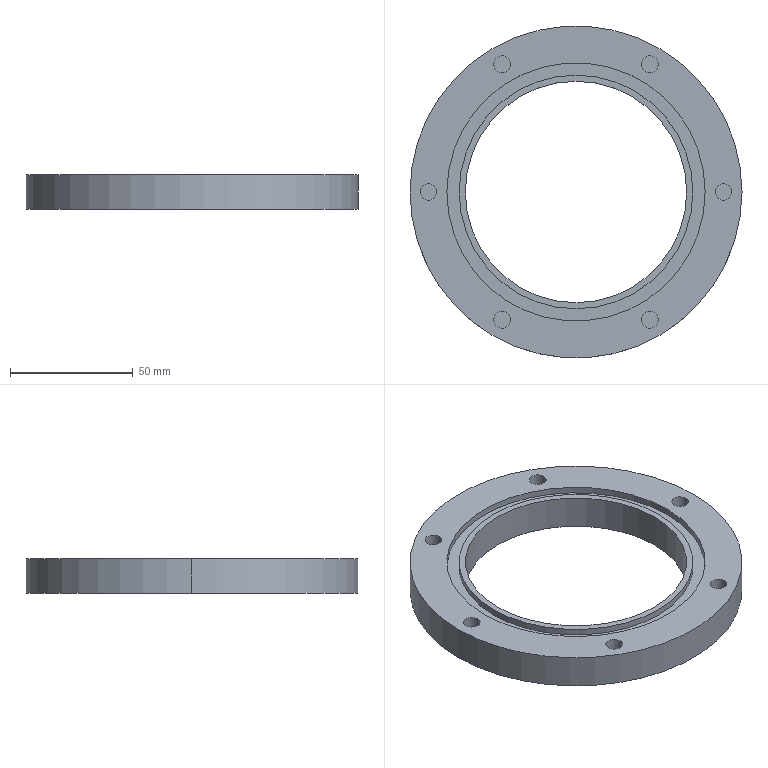Part | SolidWorks | features ICE 2, CirPattern 1, FlatPattern 1, HoleWzd 1, SMBaseFlange 1, SheetMetal 1 | 1 solid | 30 faces | box 135 x 135 x 14 mm | volume 104256 mm3 | cylinder 20 | plane 10 | commonest cylinder face diameters 6.8 x12 90 x2 95 x2 105 x2 135 x2
STEP:
#1=CARTESIAN_POINT('',(47.5,0.,-2.7));
#2=VERTEX_POINT('',#1);
#3=CARTESIAN_POINT('',(-47.5,0.,-2.7));
#4=VERTEX_POINT('',#3);
#5=CARTESIAN_POINT('',(0.,0.,-2.7));
#6=DIRECTION('',(0.,0.,1.));
#7=DIRECTION('',(1.,0.,0.));
#8=AXIS2_PLACEMENT_3D('',#5,#6,#7);
#9=CIRCLE('',#8,47.5);
#10=EDGE_CURVE('',#2,#4,#9,.T.);
#11=ORIENTED_EDGE('',*,*,#10,.T.);
#12=CARTESIAN_POINT('',(-47.5,0.,0.));
#13=VERTEX_POINT('',#12);
#14=CARTESIAN_POINT('',(-47.5,0.,-2.7));
#15=DIRECTION('',(0.,0.,1.));
#16=VECTOR('',#15,1000.);
#17=LINE('',#14,#16);
#18=EDGE_CURVE('',#4,#13,#17,.T.);
#19=ORIENTED_EDGE('',*,*,#18,.T.);
#20=CARTESIAN_POINT('',(47.5,0.,0.));
#21=VERTEX_POINT('',#20);
#22=CARTESIAN_POINT('',(0.,0.,0.));
#23=DIRECTION('',(0.,0.,1.));
#24=DIRECTION('',(1.,0.,0.));
#25=AXIS2_PLACEMENT_3D('',#22,#23,#24);
#26=CIRCLE('',#25,47.5);
#27=EDGE_CURVE('',#21,#13,#26,.T.);
#28=ORIENTED_EDGE('',*,*,#27,.F.);
#29=CARTESIAN_POINT('',(47.5,0.,-2.7));
#30=DIRECTION('',(0.,0.,1.));
#31=VECTOR('',#30,1000.);
#32=LINE('',#29,#31);
#33=EDGE_CURVE('',#2,#21,#32,.T.);
#34=ORIENTED_EDGE('',*,*,#33,.F.);
#35=EDGE_LOOP('',(#11,#19,#28,#34));
#36=FACE_OUTER_BOUND('',#35,.T.);
#37=CARTESIAN_POINT('',(0.,0.,-2.7));
#38=DIRECTION('',(0.,0.,1.));
#39=DIRECTION('',(1.,0.,0.));
#40=AXIS2_PLACEMENT_3D('',#37,#38,#39);
#41=CYLINDRICAL_SURFACE('',#40,47.5);
#42=ADVANCED_FACE('',(#36),#41,.T.);
#43=CARTESIAN_POINT('',(-52.5,0.,-2.7));
#44=VERTEX_POINT('',#43);
#45=CARTESIAN_POINT('',(52.5,0.,-2.7));
#46=VERTEX_POINT('',#45);
#47=CARTESIAN_POINT('',(0.,0.,-2.7));
#48=DIRECTION('',(0.,0.,1.));
#49=DIRECTION('',(1.,0.,0.));
#50=AXIS2_PLACEMENT_3D('',#47,#48,#49);
#51=CIRCLE('',#50,52.5);
#52=EDGE_CURVE('',#44,#46,#51,.T.);
#53=ORIENTED_EDGE('',*,*,#52,.F.);
#54=CARTESIAN_POINT('',(-52.5,0.,0.));
#55=VERTEX_POINT('',#54);
#56=CARTESIAN_POINT('',(-52.5,0.,-2.7));
#57=DIRECTION('',(0.,0.,1.));
#58=VECTOR('',#57,1000.);
#59=LINE('',#56,#58);
#60=EDGE_CURVE('',#44,#55,#59,.T.);
#61=ORIENTED_EDGE('',*,*,#60,.T.);
#62=CARTESIAN_POINT('',(52.5,0.,0.));
#63=VERTEX_POINT('',#62);
#64=CARTESIAN_POINT('',(0.,0.,0.));
#65=DIRECTION('',(0.,0.,1.));
#66=DIRECTION('',(1.,0.,0.));
#67=AXIS2_PLACEMENT_3D('',#64,#65,#66);
#68=CIRCLE('',#67,52.5);
#69=EDGE_CURVE('',#55,#63,#68,.T.);
#70=ORIENTED_EDGE('',*,*,#69,.T.);
#71=CARTESIAN_POINT('',(52.5,0.,-2.7));
#72=DIRECTION('',(0.,0.,1.));
#73=VECTOR('',#72,1000.);
#74=LINE('',#71,#73);
#75=EDGE_CURVE('',#46,#63,#74,.T.);
#76=ORIENTED_EDGE('',*,*,#75,.F.);
#77=EDGE_LOOP('',(#53,#61,#70,#76));
#78=FACE_OUTER_BOUND('',#77,.T.);
#79=CARTESIAN_POINT('',(0.,0.,-2.7));
#80=DIRECTION('',(0.,0.,1.));
#81=DIRECTION('',(1.,0.,0.));
#82=AXIS2_PLACEMENT_3D('',#79,#80,#81);
#83=CYLINDRICAL_SURFACE('',#82,52.5);
#84=ADVANCED_FACE('',(#78),#83,.F.);
#85=CARTESIAN_POINT('',(-45.,0.,-14.));
#86=VERTEX_POINT('',#85);
#87=CARTESIAN_POINT('',(45.,0.,-14.));
#88=VERTEX_POINT('',#87);
#89=CARTESIAN_POINT('',(0.,0.,-14.));
#90=DIRECTION('',(0.,0.,1.));
#91=DIRECTION('',(1.,0.,0.));
#92=AXIS2_PLACEMENT_3D('',#89,#90,#91);
#93=CIRCLE('',#92,45.);
#94=EDGE_CURVE('',#86,#88,#93,.T.);
#95=ORIENTED_EDGE('',*,*,#94,.F.);
#96=CARTESIAN_POINT('',(-45.,0.,0.));
#97=VERTEX_POINT('',#96);
#98=CARTESIAN_POINT('',(-45.,0.,-14.));
#99=DIRECTION('',(0.,0.,1.));
#100=VECTOR('',#99,1000.);
#101=LINE('',#98,#100);
#102=EDGE_CURVE('',#86,#97,#101,.T.);
#103=ORIENTED_EDGE('',*,*,#102,.T.);
#104=CARTESIAN_POINT('',(45.,0.,0.));
#105=VERTEX_POINT('',#104);
#106=CARTESIAN_POINT('',(0.,0.,0.));
#107=DIRECTION('',(0.,0.,1.));
#108=DIRECTION('',(1.,0.,0.));
#109=AXIS2_PLACEMENT_3D('',#106,#107,#108);
#110=CIRCLE('',#109,45.);
#111=EDGE_CURVE('',#97,#105,#110,.T.);
#112=ORIENTED_EDGE('',*,*,#111,.T.);
#113=CARTESIAN_POINT('',(45.,0.,-14.));
#114=DIRECTION('',(0.,0.,1.));
#115=VECTOR('',#114,1000.);
#116=LINE('',#113,#115);
#117=EDGE_CURVE('',#88,#105,#116,.T.);
#118=ORIENTED_EDGE('',*,*,#117,.F.);
#119=EDGE_LOOP('',(#95,#103,#112,#118));
#120=FACE_OUTER_BOUND('',#119,.T.);
#121=CARTESIAN_POINT('',(0.,0.,-14.));
#122=DIRECTION('',(0.,0.,1.));
#123=DIRECTION('',(1.,0.,0.));
#124=AXIS2_PLACEMENT_3D('',#121,#122,#123);
#125=CYLINDRICAL_SURFACE('',#124,45.);
#126=ADVANCED_FACE('',(#120),#125,.F.);
#127=CARTESIAN_POINT('',(67.5,0.,-14.));
#128=VERTEX_POINT('',#127);
#129=CARTESIAN_POINT('',(-67.5,0.,-14.));
#130=VERTEX_POINT('',#129);
#131=CARTESIAN_POINT('',(0.,0.,-14.));
#132=DIRECTION('',(0.,0.,1.));
#133=DIRECTION('',(1.,0.,0.));
#134=AXIS2_PLACEMENT_3D('',#131,#132,#133);
#135=CIRCLE('',#134,67.5);
#136=EDGE_CURVE('',#128,#130,#135,.T.);
#137=ORIENTED_EDGE('',*,*,#136,.T.);
#138=CARTESIAN_POINT('',(-67.5,0.,0.));
#139=VERTEX_POINT('',#138);
#140=CARTESIAN_POINT('',(-67.5,0.,-14.));
#141=DIRECTION('',(0.,0.,1.));
#142=VECTOR('',#141,1000.);
#143=LINE('',#140,#142);
#144=EDGE_CURVE('',#130,#139,#143,.T.);
#145=ORIENTED_EDGE('',*,*,#144,.T.);
#146=CARTESIAN_POINT('',(67.5,0.,0.));
#147=VERTEX_POINT('',#146);
#148=CARTESIAN_POINT('',(0.,0.,0.));
#149=DIRECTION('',(0.,0.,1.));
#150=DIRECTION('',(1.,0.,0.));
#151=AXIS2_PLACEMENT_3D('',#148,#149,#150);
#152=CIRCLE('',#151,67.5);
#153=EDGE_CURVE('',#147,#139,#152,.T.);
#154=ORIENTED_EDGE('',*,*,#153,.F.);
#155=CARTESIAN_POINT('',(67.5,0.,-14.));
#156=DIRECTION('',(0.,0.,1.));
#157=VECTOR('',#156,1000.);
#158=LINE('',#155,#157);
#159=EDGE_CURVE('',#128,#147,#158,.T.);
#160=ORIENTED_EDGE('',*,*,#159,.F.);
#161=EDGE_LOOP('',(#137,#145,#154,#160));
#162=FACE_OUTER_BOUND('',#161,.T.);
#163=CARTESIAN_POINT('',(0.,0.,-14.));
#164=DIRECTION('',(0.,0.,1.));
#165=DIRECTION('',(1.,0.,0.));
#166=AXIS2_PLACEMENT_3D('',#163,#164,#165);
#167=CYLINDRICAL_SURFACE('',#166,67.5);
#168=ADVANCED_FACE('',(#162),#167,.T.);
#169=CARTESIAN_POINT('',(26.6,-51.962,-13.));
#170=VERTEX_POINT('',#169);
#171=CARTESIAN_POINT('',(33.4,-51.962,-13.));
#172=VERTEX_POINT('',#171);
#173=CARTESIAN_POINT('',(30.,-51.962,-13.));
#174=DIRECTION('',(0.,0.,1.));
#175=DIRECTION('',(-1.,0.,0.));
#176=AXIS2_PLACEMENT_3D('',#173,#174,#175);
#177=CIRCLE('',#176,3.4);
#178=EDGE_CURVE('',#170,#172,#177,.T.);
#179=ORIENTED_EDGE('',*,*,#178,.F.);
#180=CARTESIAN_POINT('',(26.6,-51.962,0.));
#181=VERTEX_POINT('',#180);
#182=CARTESIAN_POINT('',(26.6,-51.962,0.));
#183=DIRECTION('',(0.,0.,1.));
#184=VECTOR('',#183,1000.);
#185=LINE('',#182,#184);
#186=EDGE_CURVE('',#170,#181,#185,.T.);
#187=ORIENTED_EDGE('',*,*,#186,.T.);
#188=CARTESIAN_POINT('',(33.4,-51.962,0.));
#189=VERTEX_POINT('',#188);
#190=CARTESIAN_POINT('',(30.,-51.962,0.));
#191=DIRECTION('',(0.,0.,1.));
#192=DIRECTION('',(1.,0.,0.));
#193=AXIS2_PLACEMENT_3D('',#190,#191,#192);
#194=CIRCLE('',#193,3.4);
#195=EDGE_CURVE('',#181,#189,#194,.T.);
#196=ORIENTED_EDGE('',*,*,#195,.T.);
#197=CARTESIAN_POINT('',(33.4,-51.962,0.));
#198=DIRECTION('',(0.,0.,1.));
#199=VECTOR('',#198,1000.);
#200=LINE('',#197,#199);
#201=EDGE_CURVE('',#172,#189,#200,.T.);
#202=ORIENTED_EDGE('',*,*,#201,.F.);
#203=EDGE_LOOP('',(#179,#187,#196,#202));
#204=FACE_OUTER_BOUND('',#203,.T.);
#205=CARTESIAN_POINT('',(30.,-51.962,0.));
#206=DIRECTION('',(0.,0.,1.));
#207=DIRECTION('',(1.,0.,0.));
#208=AXIS2_PLACEMENT_3D('',#205,#206,#207);
#209=CYLINDRICAL_SURFACE('',#208,3.4);
#210=ADVANCED_FACE('',(#204),#209,.F.);
#211=CARTESIAN_POINT('',(-33.4,-51.962,-13.));
#212=VERTEX_POINT('',#211);
#213=CARTESIAN_POINT('',(-26.6,-51.962,-13.));
#214=VERTEX_POINT('',#213);
#215=CARTESIAN_POINT('',(-30.,-51.962,-13.));
#216=DIRECTION('',(0.,0.,1.));
#217=DIRECTION('',(-1.,0.,0.));
#218=AXIS2_PLACEMENT_3D('',#215,#216,#217);
#219=CIRCLE('',#218,3.4);
#220=EDGE_CURVE('',#212,#214,#219,.T.);
#221=ORIENTED_EDGE('',*,*,#220,.F.);
#222=CARTESIAN_POINT('',(-33.4,-51.962,0.));
#223=VERTEX_POINT('',#222);
#224=CARTESIAN_POINT('',(-33.4,-51.962,0.));
#225=DIRECTION('',(0.,0.,1.));
#226=VECTOR('',#225,1000.);
#227=LINE('',#224,#226);
#228=EDGE_CURVE('',#212,#223,#227,.T.);
#229=ORIENTED_EDGE('',*,*,#228,.T.);
#230=CARTESIAN_POINT('',(-26.6,-51.962,0.));
#231=VERTEX_POINT('',#230);
#232=CARTESIAN_POINT('',(-30.,-51.962,0.));
#233=DIRECTION('',(0.,0.,1.));
#234=DIRECTION('',(1.,0.,0.));
#235=AXIS2_PLACEMENT_3D('',#232,#233,#234);
#236=CIRCLE('',#235,3.4);
#237=EDGE_CURVE('',#223,#231,#236,.T.);
#238=ORIENTED_EDGE('',*,*,#237,.T.);
#239=CARTESIAN_POINT('',(-26.6,-51.962,0.));
#240=DIRECTION('',(0.,0.,1.));
#241=VECTOR('',#240,1000.);
#242=LINE('',#239,#241);
#243=EDGE_CURVE('',#214,#231,#242,.T.);
#244=ORIENTED_EDGE('',*,*,#243,.F.);
#245=EDGE_LOOP('',(#221,#229,#238,#244));
#246=FACE_OUTER_BOUND('',#245,.T.);
#247=CARTESIAN_POINT('',(-30.,-51.962,0.));
#248=DIRECTION('',(0.,0.,1.));
#249=DIRECTION('',(1.,0.,0.));
#250=AXIS2_PLACEMENT_3D('',#247,#248,#249);
#251=CYLINDRICAL_SURFACE('',#250,3.4);
#252=ADVANCED_FACE('',(#246),#251,.F.);
#253=CARTESIAN_POINT('',(-63.4,0.,-13.));
#254=VERTEX_POINT('',#253);
#255=CARTESIAN_POINT('',(-56.6,0.,-13.));
#256=VERTEX_POINT('',#255);
#257=CARTESIAN_POINT('',(-60.,0.,-13.));
#258=DIRECTION('',(0.,0.,1.));
#259=DIRECTION('',(-1.,0.,0.));
#260=AXIS2_PLACEMENT_3D('',#257,#258,#259);
#261=CIRCLE('',#260,3.4);
#262=EDGE_CURVE('',#254,#256,#261,.T.);
#263=ORIENTED_EDGE('',*,*,#262,.F.);
#264=CARTESIAN_POINT('',(-63.4,0.,0.));
#265=VERTEX_POINT('',#264);
#266=CARTESIAN_POINT('',(-63.4,0.,0.));
#267=DIRECTION('',(0.,0.,1.));
#268=VECTOR('',#267,1000.);
#269=LINE('',#266,#268);
#270=EDGE_CURVE('',#254,#265,#269,.T.);
#271=ORIENTED_EDGE('',*,*,#270,.T.);
#272=CARTESIAN_POINT('',(-56.6,0.,0.));
#273=VERTEX_POINT('',#272);
#274=CARTESIAN_POINT('',(-60.,0.,0.));
#275=DIRECTION('',(0.,0.,1.));
#276=DIRECTION('',(1.,0.,0.));
#277=AXIS2_PLACEMENT_3D('',#274,#275,#276);
#278=CIRCLE('',#277,3.4);
#279=EDGE_CURVE('',#265,#273,#278,.T.);
#280=ORIENTED_EDGE('',*,*,#279,.T.);
#281=CARTESIAN_POINT('',(-56.6,0.,0.));
#282=DIRECTION('',(0.,0.,1.));
#283=VECTOR('',#282,1000.);
#284=LINE('',#281,#283);
#285=EDGE_CURVE('',#256,#273,#284,.T.);
#286=ORIENTED_EDGE('',*,*,#285,.F.);
#287=EDGE_LOOP('',(#263,#271,#280,#286));
#288=FACE_OUTER_BOUND('',#287,.T.);
#289=CARTESIAN_POINT('',(-60.,0.,0.));
#290=DIRECTION('',(0.,0.,1.));
#291=DIRECTION('',(1.,0.,0.));
#292=AXIS2_PLACEMENT_3D('',#289,#290,#291);
#293=CYLINDRICAL_SURFACE('',#292,3.4);
#294=ADVANCED_FACE('',(#288),#293,.F.);
#295=CARTESIAN_POINT('',(-33.4,51.962,-13.));
#296=VERTEX_POINT('',#295);
#297=CARTESIAN_POINT('',(-26.6,51.962,-13.));
#298=VERTEX_POINT('',#297);
#299=CARTESIAN_POINT('',(-30.,51.962,-13.));
#300=DIRECTION('',(0.,0.,1.));
#301=DIRECTION('',(-1.,0.,0.));
#302=AXIS2_PLACEMENT_3D('',#299,#300,#301);
#303=CIRCLE('',#302,3.4);
#304=EDGE_CURVE('',#296,#298,#303,.T.);
#305=ORIENTED_EDGE('',*,*,#304,.F.);
#306=CARTESIAN_POINT('',(-33.4,51.962,0.));
#307=VERTEX_POINT('',#306);
#308=CARTESIAN_POINT('',(-33.4,51.962,0.));
#309=DIRECTION('',(0.,0.,1.));
#310=VECTOR('',#309,1000.);
#311=LINE('',#308,#310);
#312=EDGE_CURVE('',#296,#307,#311,.T.);
#313=ORIENTED_EDGE('',*,*,#312,.T.);
#314=CARTESIAN_POINT('',(-26.6,51.962,0.));
#315=VERTEX_POINT('',#314);
#316=CARTESIAN_POINT('',(-30.,51.962,0.));
#317=DIRECTION('',(0.,0.,1.));
#318=DIRECTION('',(1.,0.,0.));
#319=AXIS2_PLACEMENT_3D('',#316,#317,#318);
#320=CIRCLE('',#319,3.4);
#321=EDGE_CURVE('',#307,#315,#320,.T.);
#322=ORIENTED_EDGE('',*,*,#321,.T.);
#323=CARTESIAN_POINT('',(-26.6,51.962,0.));
#324=DIRECTION('',(0.,0.,1.));
#325=VECTOR('',#324,1000.);
#326=LINE('',#323,#325);
#327=EDGE_CURVE('',#298,#315,#326,.T.);
#328=ORIENTED_EDGE('',*,*,#327,.F.);
#329=EDGE_LOOP('',(#305,#313,#322,#328));
#330=FACE_OUTER_BOUND('',#329,.T.);
#331=CARTESIAN_POINT('',(-30.,51.962,0.));
#332=DIRECTION('',(0.,0.,1.));
#333=DIRECTION('',(1.,0.,0.));
#334=AXIS2_PLACEMENT_3D('',#331,#332,#333);
#335=CYLINDRICAL_SURFACE('',#334,3.4);
#336=ADVANCED_FACE('',(#330),#335,.F.);
#337=CARTESIAN_POINT('',(26.6,51.962,-13.));
#338=VERTEX_POINT('',#337);
#339=CARTESIAN_POINT('',(33.4,51.962,-13.));
#340=VERTEX_POINT('',#339);
#341=CARTESIAN_POINT('',(30.,51.962,-13.));
#342=DIRECTION('',(0.,0.,1.));
#343=DIRECTION('',(-1.,0.,0.));
#344=AXIS2_PLACEMENT_3D('',#341,#342,#343);
#345=CIRCLE('',#344,3.4);
#346=EDGE_CURVE('',#338,#340,#345,.T.);
#347=ORIENTED_EDGE('',*,*,#346,.F.);
#348=CARTESIAN_POINT('',(26.6,51.962,0.));
#349=VERTEX_POINT('',#348);
#350=CARTESIAN_POINT('',(26.6,51.962,0.));
#351=DIRECTION('',(0.,0.,1.));
#352=VECTOR('',#351,1000.);
#353=LINE('',#350,#352);
#354=EDGE_CURVE('',#338,#349,#353,.T.);
#355=ORIENTED_EDGE('',*,*,#354,.T.);
#356=CARTESIAN_POINT('',(33.4,51.962,0.));
#357=VERTEX_POINT('',#356);
#358=CARTESIAN_POINT('',(30.,51.962,0.));
#359=DIRECTION('',(0.,0.,1.));
#360=DIRECTION('',(1.,0.,0.));
#361=AXIS2_PLACEMENT_3D('',#358,#359,#360);
#362=CIRCLE('',#361,3.4);
#363=EDGE_CURVE('',#349,#357,#362,.T.);
#364=ORIENTED_EDGE('',*,*,#363,.T.);
#365=CARTESIAN_POINT('',(33.4,51.962,0.));
#366=DIRECTION('',(0.,0.,1.));
#367=VECTOR('',#366,1000.);
#368=LINE('',#365,#367);
#369=EDGE_CURVE('',#340,#357,#368,.T.);
#370=ORIENTED_EDGE('',*,*,#369,.F.);
#371=EDGE_LOOP('',(#347,#355,#364,#370));
#372=FACE_OUTER_BOUND('',#371,.T.);
#373=CARTESIAN_POINT('',(30.,51.962,0.));
#374=DIRECTION('',(0.,0.,1.));
#375=DIRECTION('',(1.,0.,0.));
#376=AXIS2_PLACEMENT_3D('',#373,#374,#375);
#377=CYLINDRICAL_SURFACE('',#376,3.4);
#378=ADVANCED_FACE('',(#372),#377,.F.);
#379=CARTESIAN_POINT('',(56.6,0.,-13.));
#380=VERTEX_POINT('',#379);
#381=CARTESIAN_POINT('',(63.4,0.,-13.));
#382=VERTEX_POINT('',#381);
#383=CARTESIAN_POINT('',(60.,0.,-13.));
#384=DIRECTION('',(0.,0.,1.));
#385=DIRECTION('',(-1.,0.,0.));
#386=AXIS2_PLACEMENT_3D('',#383,#384,#385);
#387=CIRCLE('',#386,3.4);
#388=EDGE_CURVE('',#380,#382,#387,.T.);
#389=ORIENTED_EDGE('',*,*,#388,.F.);
#390=CARTESIAN_POINT('',(56.6,0.,0.));
#391=VERTEX_POINT('',#390);
#392=CARTESIAN_POINT('',(56.6,0.,0.));
#393=DIRECTION('',(0.,0.,1.));
#394=VECTOR('',#393,1000.);
#395=LINE('',#392,#394);
#396=EDGE_CURVE('',#380,#391,#395,.T.);
#397=ORIENTED_EDGE('',*,*,#396,.T.);
#398=CARTESIAN_POINT('',(63.4,0.,0.));
#399=VERTEX_POINT('',#398);
#400=CARTESIAN_POINT('',(60.,0.,0.));
#401=DIRECTION('',(0.,0.,1.));
#402=DIRECTION('',(1.,0.,0.));
#403=AXIS2_PLACEMENT_3D('',#400,#401,#402);
#404=CIRCLE('',#403,3.4);
#405=EDGE_CURVE('',#391,#399,#404,.T.);
#406=ORIENTED_EDGE('',*,*,#405,.T.);
#407=CARTESIAN_POINT('',(63.4,0.,0.));
#408=DIRECTION('',(0.,0.,1.));
#409=VECTOR('',#408,1000.);
#410=LINE('',#407,#409);
#411=EDGE_CURVE('',#382,#399,#410,.T.);
#412=ORIENTED_EDGE('',*,*,#411,.F.);
#413=EDGE_LOOP('',(#389,#397,#406,#412));
#414=FACE_OUTER_BOUND('',#413,.T.);
#415=CARTESIAN_POINT('',(60.,0.,0.));
#416=DIRECTION('',(0.,0.,1.));
#417=DIRECTION('',(1.,0.,0.));
#418=AXIS2_PLACEMENT_3D('',#415,#416,#417);
#419=CYLINDRICAL_SURFACE('',#418,3.4);
#420=ADVANCED_FACE('',(#414),#419,.F.);
#421=ORIENTED_EDGE('',*,*,#396,.F.);
#422=CARTESIAN_POINT('',(60.,0.,-13.));
#423=DIRECTION('',(0.,0.,1.));
#424=DIRECTION('',(-1.,0.,0.));
#425=AXIS2_PLACEMENT_3D('',#422,#423,#424);
#426=CIRCLE('',#425,3.4);
#427=EDGE_CURVE('',#382,#380,#426,.T.);
#428=ORIENTED_EDGE('',*,*,#427,.F.);
#429=ORIENTED_EDGE('',*,*,#411,.T.);
#430=CARTESIAN_POINT('',(60.,0.,0.));
#431=DIRECTION('',(0.,0.,1.));
#432=DIRECTION('',(1.,0.,0.));
#433=AXIS2_PLACEMENT_3D('',#430,#431,#432);
#434=CIRCLE('',#433,3.4);
#435=EDGE_CURVE('',#399,#391,#434,.T.);
#436=ORIENTED_EDGE('',*,*,#435,.T.);
#437=EDGE_LOOP('',(#421,#428,#429,#436));
#438=FACE_OUTER_BOUND('',#437,.T.);
#439=CARTESIAN_POINT('',(60.,0.,0.));
#440=DIRECTION('',(0.,0.,1.));
#441=DIRECTION('',(1.,0.,0.));
#442=AXIS2_PLACEMENT_3D('',#439,#440,#441);
#443=CYLINDRICAL_SURFACE('',#442,3.4);
#444=ADVANCED_FACE('',(#438),#443,.F.);
#445=ORIENTED_EDGE('',*,*,#354,.F.);
#446=CARTESIAN_POINT('',(30.,51.962,-13.));
#447=DIRECTION('',(0.,0.,1.));
#448=DIRECTION('',(-1.,0.,0.));
#449=AXIS2_PLACEMENT_3D('',#446,#447,#448);
#450=CIRCLE('',#449,3.4);
#451=EDGE_CURVE('',#340,#338,#450,.T.);
#452=ORIENTED_EDGE('',*,*,#451,.F.);
#453=ORIENTED_EDGE('',*,*,#369,.T.);
#454=CARTESIAN_POINT('',(30.,51.962,0.));
#455=DIRECTION('',(0.,0.,1.));
#456=DIRECTION('',(1.,0.,0.));
#457=AXIS2_PLACEMENT_3D('',#454,#455,#456);
#458=CIRCLE('',#457,3.4);
#459=EDGE_CURVE('',#357,#349,#458,.T.);
#460=ORIENTED_EDGE('',*,*,#459,.T.);
#461=EDGE_LOOP('',(#445,#452,#453,#460));
#462=FACE_OUTER_BOUND('',#461,.T.);
#463=CARTESIAN_POINT('',(30.,51.962,0.));
#464=DIRECTION('',(0.,0.,1.));
#465=DIRECTION('',(1.,0.,0.));
#466=AXIS2_PLACEMENT_3D('',#463,#464,#465);
#467=CYLINDRICAL_SURFACE('',#466,3.4);
#468=ADVANCED_FACE('',(#462),#467,.F.);
#469=ORIENTED_EDGE('',*,*,#312,.F.);
#470=CARTESIAN_POINT('',(-30.,51.962,-13.));
#471=DIRECTION('',(0.,0.,1.));
#472=DIRECTION('',(-1.,0.,0.));
#473=AXIS2_PLACEMENT_3D('',#470,#471,#472);
#474=CIRCLE('',#473,3.4);
#475=EDGE_CURVE('',#298,#296,#474,.T.);
#476=ORIENTED_EDGE('',*,*,#475,.F.);
#477=ORIENTED_EDGE('',*,*,#327,.T.);
#478=CARTESIAN_POINT('',(-30.,51.962,0.));
#479=DIRECTION('',(0.,0.,1.));
#480=DIRECTION('',(1.,0.,0.));
#481=AXIS2_PLACEMENT_3D('',#478,#479,#480);
#482=CIRCLE('',#481,3.4);
#483=EDGE_CURVE('',#315,#307,#482,.T.);
#484=ORIENTED_EDGE('',*,*,#483,.T.);
#485=EDGE_LOOP('',(#469,#476,#477,#484));
#486=FACE_OUTER_BOUND('',#485,.T.);
#487=CARTESIAN_POINT('',(-30.,51.962,0.));
#488=DIRECTION('',(0.,0.,1.));
#489=DIRECTION('',(1.,0.,0.));
#490=AXIS2_PLACEMENT_3D('',#487,#488,#489);
#491=CYLINDRICAL_SURFACE('',#490,3.4);
#492=ADVANCED_FACE('',(#486),#491,.F.);
#493=ORIENTED_EDGE('',*,*,#270,.F.);
#494=CARTESIAN_POINT('',(-60.,0.,-13.));
#495=DIRECTION('',(0.,0.,1.));
#496=DIRECTION('',(-1.,0.,0.));
#497=AXIS2_PLACEMENT_3D('',#494,#495,#496);
#498=CIRCLE('',#497,3.4);
#499=EDGE_CURVE('',#256,#254,#498,.T.);
#500=ORIENTED_EDGE('',*,*,#499,.F.);
#501=ORIENTED_EDGE('',*,*,#285,.T.);
#502=CARTESIAN_POINT('',(-60.,0.,0.));
#503=DIRECTION('',(0.,0.,1.));
#504=DIRECTION('',(1.,0.,0.));
#505=AXIS2_PLACEMENT_3D('',#502,#503,#504);
#506=CIRCLE('',#505,3.4);
#507=EDGE_CURVE('',#273,#265,#506,.T.);
#508=ORIENTED_EDGE('',*,*,#507,.T.);
#509=EDGE_LOOP('',(#493,#500,#501,#508));
#510=FACE_OUTER_BOUND('',#509,.T.);
#511=CARTESIAN_POINT('',(-60.,0.,0.));
#512=DIRECTION('',(0.,0.,1.));
#513=DIRECTION('',(1.,0.,0.));
#514=AXIS2_PLACEMENT_3D('',#511,#512,#513);
#515=CYLINDRICAL_SURFACE('',#514,3.4);
#516=ADVANCED_FACE('',(#510),#515,.F.);
#517=ORIENTED_EDGE('',*,*,#228,.F.);
#518=CARTESIAN_POINT('',(-30.,-51.962,-13.));
#519=DIRECTION('',(0.,0.,1.));
#520=DIRECTION('',(-1.,0.,0.));
#521=AXIS2_PLACEMENT_3D('',#518,#519,#520);
#522=CIRCLE('',#521,3.4);
#523=EDGE_CURVE('',#214,#212,#522,.T.);
#524=ORIENTED_EDGE('',*,*,#523,.F.);
#525=ORIENTED_EDGE('',*,*,#243,.T.);
#526=CARTESIAN_POINT('',(-30.,-51.962,0.));
#527=DIRECTION('',(0.,0.,1.));
#528=DIRECTION('',(1.,0.,0.));
#529=AXIS2_PLACEMENT_3D('',#526,#527,#528);
#530=CIRCLE('',#529,3.4);
#531=EDGE_CURVE('',#231,#223,#530,.T.);
#532=ORIENTED_EDGE('',*,*,#531,.T.);
#533=EDGE_LOOP('',(#517,#524,#525,#532));
#534=FACE_OUTER_BOUND('',#533,.T.);
#535=CARTESIAN_POINT('',(-30.,-51.962,0.));
#536=DIRECTION('',(0.,0.,1.));
#537=DIRECTION('',(1.,0.,0.));
#538=AXIS2_PLACEMENT_3D('',#535,#536,#537);
#539=CYLINDRICAL_SURFACE('',#538,3.4);
#540=ADVANCED_FACE('',(#534),#539,.F.);
#541=ORIENTED_EDGE('',*,*,#186,.F.);
#542=CARTESIAN_POINT('',(30.,-51.962,-13.));
#543=DIRECTION('',(0.,0.,1.));
#544=DIRECTION('',(-1.,0.,0.));
#545=AXIS2_PLACEMENT_3D('',#542,#543,#544);
#546=CIRCLE('',#545,3.4);
#547=EDGE_CURVE('',#172,#170,#546,.T.);
#548=ORIENTED_EDGE('',*,*,#547,.F.);
#549=ORIENTED_EDGE('',*,*,#201,.T.);
#550=CARTESIAN_POINT('',(30.,-51.962,0.));
#551=DIRECTION('',(0.,0.,1.));
#552=DIRECTION('',(1.,0.,0.));
#553=AXIS2_PLACEMENT_3D('',#550,#551,#552);
#554=CIRCLE('',#553,3.4);
#555=EDGE_CURVE('',#189,#181,#554,.T.);
#556=ORIENTED_EDGE('',*,*,#555,.T.);
#557=EDGE_LOOP('',(#541,#548,#549,#556));
#558=FACE_OUTER_BOUND('',#557,.T.);
#559=CARTESIAN_POINT('',(30.,-51.962,0.));
#560=DIRECTION('',(0.,0.,1.));
#561=DIRECTION('',(1.,0.,0.));
#562=AXIS2_PLACEMENT_3D('',#559,#560,#561);
#563=CYLINDRICAL_SURFACE('',#562,3.4);
#564=ADVANCED_FACE('',(#558),#563,.F.);
#565=CARTESIAN_POINT('',(0.,0.,0.));
#566=DIRECTION('',(0.,0.,1.));
#567=DIRECTION('',(1.,0.,0.));
#568=AXIS2_PLACEMENT_3D('',#565,#566,#567);
#569=CIRCLE('',#568,45.);
#570=EDGE_CURVE('',#105,#97,#569,.T.);
#571=ORIENTED_EDGE('',*,*,#570,.F.);
#572=ORIENTED_EDGE('',*,*,#111,.F.);
#573=EDGE_LOOP('',(#571,#572));
#574=FACE_BOUND('',#573,.T.);
#575=ORIENTED_EDGE('',*,*,#27,.T.);
#576=CARTESIAN_POINT('',(0.,0.,0.));
#577=DIRECTION('',(0.,0.,1.));
#578=DIRECTION('',(1.,0.,0.));
#579=AXIS2_PLACEMENT_3D('',#576,#577,#578);
#580=CIRCLE('',#579,47.5);
#581=EDGE_CURVE('',#13,#21,#580,.T.);
#582=ORIENTED_EDGE('',*,*,#581,.T.);
#583=EDGE_LOOP('',(#575,#582));
#584=FACE_OUTER_BOUND('',#583,.T.);
#585=CARTESIAN_POINT('',(0.,0.,0.));
#586=DIRECTION('',(0.,0.,1.));
#587=DIRECTION('',(1.,0.,0.));
#588=AXIS2_PLACEMENT_3D('',#585,#586,#587);
#589=PLANE('',#588);
#590=ADVANCED_FACE('',(#574,#584),#589,.T.);
#591=ORIENTED_EDGE('',*,*,#144,.F.);
#592=CARTESIAN_POINT('',(0.,0.,-14.));
#593=DIRECTION('',(0.,0.,1.));
#594=DIRECTION('',(1.,0.,0.));
#595=AXIS2_PLACEMENT_3D('',#592,#593,#594);
#596=CIRCLE('',#595,67.5);
#597=EDGE_CURVE('',#130,#128,#596,.T.);
#598=ORIENTED_EDGE('',*,*,#597,.T.);
#599=ORIENTED_EDGE('',*,*,#159,.T.);
#600=CARTESIAN_POINT('',(0.,0.,0.));
#601=DIRECTION('',(0.,0.,1.));
#602=DIRECTION('',(1.,0.,0.));
#603=AXIS2_PLACEMENT_3D('',#600,#601,#602);
#604=CIRCLE('',#603,67.5);
#605=EDGE_CURVE('',#139,#147,#604,.T.);
#606=ORIENTED_EDGE('',*,*,#605,.F.);
#607=EDGE_LOOP('',(#591,#598,#599,#606));
#608=FACE_OUTER_BOUND('',#607,.T.);
#609=CARTESIAN_POINT('',(0.,0.,-14.));
#610=DIRECTION('',(0.,0.,1.));
#611=DIRECTION('',(1.,0.,0.));
#612=AXIS2_PLACEMENT_3D('',#609,#610,#611);
#613=CYLINDRICAL_SURFACE('',#612,67.5);
#614=ADVANCED_FACE('',(#608),#613,.T.);
#615=CARTESIAN_POINT('',(0.,0.,-14.));
#616=DIRECTION('',(0.,0.,1.));
#617=DIRECTION('',(1.,0.,0.));
#618=AXIS2_PLACEMENT_3D('',#615,#616,#617);
#619=CIRCLE('',#618,45.);
#620=EDGE_CURVE('',#88,#86,#619,.T.);
#621=ORIENTED_EDGE('',*,*,#620,.T.);
#622=ORIENTED_EDGE('',*,*,#94,.T.);
#623=EDGE_LOOP('',(#621,#622));
#624=FACE_BOUND('',#623,.T.);
#625=ORIENTED_EDGE('',*,*,#136,.F.);
#626=ORIENTED_EDGE('',*,*,#597,.F.);
#627=EDGE_LOOP('',(#625,#626));
#628=FACE_OUTER_BOUND('',#627,.T.);
#629=CARTESIAN_POINT('',(0.,0.,-14.));
#630=DIRECTION('',(0.,0.,1.));
#631=DIRECTION('',(1.,0.,0.));
#632=AXIS2_PLACEMENT_3D('',#629,#630,#631);
#633=PLANE('',#632);
#634=ADVANCED_FACE('',(#624,#628),#633,.F.);
#635=ORIENTED_EDGE('',*,*,#555,.F.);
#636=ORIENTED_EDGE('',*,*,#195,.F.);
#637=EDGE_LOOP('',(#635,#636));
#638=FACE_BOUND('',#637,.T.);
#639=ORIENTED_EDGE('',*,*,#531,.F.);
#640=ORIENTED_EDGE('',*,*,#237,.F.);
#641=EDGE_LOOP('',(#639,#640));
#642=FACE_BOUND('',#641,.T.);
#643=ORIENTED_EDGE('',*,*,#507,.F.);
#644=ORIENTED_EDGE('',*,*,#279,.F.);
#645=EDGE_LOOP('',(#643,#644));
#646=FACE_BOUND('',#645,.T.);
#647=ORIENTED_EDGE('',*,*,#483,.F.);
#648=ORIENTED_EDGE('',*,*,#321,.F.);
#649=EDGE_LOOP('',(#647,#648));
#650=FACE_BOUND('',#649,.T.);
#651=ORIENTED_EDGE('',*,*,#459,.F.);
#652=ORIENTED_EDGE('',*,*,#363,.F.);
#653=EDGE_LOOP('',(#651,#652));
#654=FACE_BOUND('',#653,.T.);
#655=ORIENTED_EDGE('',*,*,#435,.F.);
#656=ORIENTED_EDGE('',*,*,#405,.F.);
#657=EDGE_LOOP('',(#655,#656));
#658=FACE_BOUND('',#657,.T.);
#659=CARTESIAN_POINT('',(0.,0.,0.));
#660=DIRECTION('',(0.,0.,1.));
#661=DIRECTION('',(1.,0.,0.));
#662=AXIS2_PLACEMENT_3D('',#659,#660,#661);
#663=CIRCLE('',#662,52.5);
#664=EDGE_CURVE('',#63,#55,#663,.T.);
#665=ORIENTED_EDGE('',*,*,#664,.F.);
#666=ORIENTED_EDGE('',*,*,#69,.F.);
#667=EDGE_LOOP('',(#665,#666));
#668=FACE_BOUND('',#667,.T.);
#669=ORIENTED_EDGE('',*,*,#153,.T.);
#670=ORIENTED_EDGE('',*,*,#605,.T.);
#671=EDGE_LOOP('',(#669,#670));
#672=FACE_OUTER_BOUND('',#671,.T.);
#673=CARTESIAN_POINT('',(0.,0.,0.));
#674=DIRECTION('',(0.,0.,1.));
#675=DIRECTION('',(1.,0.,0.));
#676=AXIS2_PLACEMENT_3D('',#673,#674,#675);
#677=PLANE('',#676);
#678=ADVANCED_FACE('',(#638,#642,#646,#650,#654,#658,#668,#672),#677,.T.);
#679=ORIENTED_EDGE('',*,*,#102,.F.);
#680=ORIENTED_EDGE('',*,*,#620,.F.);
#681=ORIENTED_EDGE('',*,*,#117,.T.);
#682=ORIENTED_EDGE('',*,*,#570,.T.);
#683=EDGE_LOOP('',(#679,#680,#681,#682));
#684=FACE_OUTER_BOUND('',#683,.T.);
#685=CARTESIAN_POINT('',(0.,0.,-14.));
#686=DIRECTION('',(0.,0.,1.));
#687=DIRECTION('',(1.,0.,0.));
#688=AXIS2_PLACEMENT_3D('',#685,#686,#687);
#689=CYLINDRICAL_SURFACE('',#688,45.);
#690=ADVANCED_FACE('',(#684),#689,.F.);
#691=ORIENTED_EDGE('',*,*,#60,.F.);
#692=CARTESIAN_POINT('',(0.,0.,-2.7));
#693=DIRECTION('',(0.,0.,1.));
#694=DIRECTION('',(1.,0.,0.));
#695=AXIS2_PLACEMENT_3D('',#692,#693,#694);
#696=CIRCLE('',#695,52.5);
#697=EDGE_CURVE('',#46,#44,#696,.T.);
#698=ORIENTED_EDGE('',*,*,#697,.F.);
#699=ORIENTED_EDGE('',*,*,#75,.T.);
#700=ORIENTED_EDGE('',*,*,#664,.T.);
#701=EDGE_LOOP('',(#691,#698,#699,#700));
#702=FACE_OUTER_BOUND('',#701,.T.);
#703=CARTESIAN_POINT('',(0.,0.,-2.7));
#704=DIRECTION('',(0.,0.,1.));
#705=DIRECTION('',(1.,0.,0.));
#706=AXIS2_PLACEMENT_3D('',#703,#704,#705);
#707=CYLINDRICAL_SURFACE('',#706,52.5);
#708=ADVANCED_FACE('',(#702),#707,.F.);
#709=ORIENTED_EDGE('',*,*,#10,.F.);
#710=CARTESIAN_POINT('',(0.,0.,-2.7));
#711=DIRECTION('',(0.,0.,1.));
#712=DIRECTION('',(1.,0.,0.));
#713=AXIS2_PLACEMENT_3D('',#710,#711,#712);
#714=CIRCLE('',#713,47.5);
#715=EDGE_CURVE('',#4,#2,#714,.T.);
#716=ORIENTED_EDGE('',*,*,#715,.F.);
#717=EDGE_LOOP('',(#709,#716));
#718=FACE_BOUND('',#717,.T.);
#719=ORIENTED_EDGE('',*,*,#697,.T.);
#720=ORIENTED_EDGE('',*,*,#52,.T.);
#721=EDGE_LOOP('',(#719,#720));
#722=FACE_OUTER_BOUND('',#721,.T.);
#723=CARTESIAN_POINT('',(0.,0.,-2.7));
#724=DIRECTION('',(0.,0.,1.));
#725=DIRECTION('',(1.,0.,0.));
#726=AXIS2_PLACEMENT_3D('',#723,#724,#725);
#727=PLANE('',#726);
#728=ADVANCED_FACE('',(#718,#722),#727,.T.);
#729=ORIENTED_EDGE('',*,*,#18,.F.);
#730=ORIENTED_EDGE('',*,*,#715,.T.);
#731=ORIENTED_EDGE('',*,*,#33,.T.);
#732=ORIENTED_EDGE('',*,*,#581,.F.);
#733=EDGE_LOOP('',(#729,#730,#731,#732));
#734=FACE_OUTER_BOUND('',#733,.T.);
#735=CARTESIAN_POINT('',(0.,0.,-2.7));
#736=DIRECTION('',(0.,0.,1.));
#737=DIRECTION('',(1.,0.,0.));
#738=AXIS2_PLACEMENT_3D('',#735,#736,#737);
#739=CYLINDRICAL_SURFACE('',#738,47.5);
#740=ADVANCED_FACE('',(#734),#739,.T.);
#741=ORIENTED_EDGE('',*,*,#547,.T.);
#742=ORIENTED_EDGE('',*,*,#178,.T.);
#743=EDGE_LOOP('',(#741,#742));
#744=FACE_OUTER_BOUND('',#743,.T.);
#745=CARTESIAN_POINT('',(0.,0.,-13.));
#746=DIRECTION('',(0.,0.,-1.));
#747=DIRECTION('',(-1.,0.,0.));
#748=AXIS2_PLACEMENT_3D('',#745,#746,#747);
#749=PLANE('',#748);
#750=ADVANCED_FACE('',(#744),#749,.F.);
#751=ORIENTED_EDGE('',*,*,#523,.T.);
#752=ORIENTED_EDGE('',*,*,#220,.T.);
#753=EDGE_LOOP('',(#751,#752));
#754=FACE_OUTER_BOUND('',#753,.T.);
#755=CARTESIAN_POINT('',(0.,0.,-13.));
#756=DIRECTION('',(0.,0.,-1.));
#757=DIRECTION('',(-1.,0.,0.));
#758=AXIS2_PLACEMENT_3D('',#755,#756,#757);
#759=PLANE('',#758);
#760=ADVANCED_FACE('',(#754),#759,.F.);
#761=ORIENTED_EDGE('',*,*,#499,.T.);
#762=ORIENTED_EDGE('',*,*,#262,.T.);
#763=EDGE_LOOP('',(#761,#762));
#764=FACE_OUTER_BOUND('',#763,.T.);
#765=CARTESIAN_POINT('',(0.,0.,-13.));
#766=DIRECTION('',(0.,0.,-1.));
#767=DIRECTION('',(-1.,0.,0.));
#768=AXIS2_PLACEMENT_3D('',#765,#766,#767);
#769=PLANE('',#768);
#770=ADVANCED_FACE('',(#764),#769,.F.);
#771=ORIENTED_EDGE('',*,*,#475,.T.);
#772=ORIENTED_EDGE('',*,*,#304,.T.);
#773=EDGE_LOOP('',(#771,#772));
#774=FACE_OUTER_BOUND('',#773,.T.);
#775=CARTESIAN_POINT('',(0.,0.,-13.));
#776=DIRECTION('',(0.,0.,-1.));
#777=DIRECTION('',(-1.,0.,0.));
#778=AXIS2_PLACEMENT_3D('',#775,#776,#777);
#779=PLANE('',#778);
#780=ADVANCED_FACE('',(#774),#779,.F.);
#781=ORIENTED_EDGE('',*,*,#451,.T.);
#782=ORIENTED_EDGE('',*,*,#346,.T.);
#783=EDGE_LOOP('',(#781,#782));
#784=FACE_OUTER_BOUND('',#783,.T.);
#785=CARTESIAN_POINT('',(0.,0.,-13.));
#786=DIRECTION('',(0.,0.,-1.));
#787=DIRECTION('',(-1.,0.,0.));
#788=AXIS2_PLACEMENT_3D('',#785,#786,#787);
#789=PLANE('',#788);
#790=ADVANCED_FACE('',(#784),#789,.F.);
#791=ORIENTED_EDGE('',*,*,#427,.T.);
#792=ORIENTED_EDGE('',*,*,#388,.T.);
#793=EDGE_LOOP('',(#791,#792));
#794=FACE_OUTER_BOUND('',#793,.T.);
#795=CARTESIAN_POINT('',(0.,0.,-13.));
#796=DIRECTION('',(0.,0.,-1.));
#797=DIRECTION('',(-1.,0.,0.));
#798=AXIS2_PLACEMENT_3D('',#795,#796,#797);
#799=PLANE('',#798);
#800=ADVANCED_FACE('',(#794),#799,.F.);
#801=CLOSED_SHELL('',(#42,#84,#126,#168,#210,#252,#294,#336,#378,#420,#444,#468,#492,#516,#540,#564,#590,#614,#634,#678,#690,#708,#728,#740,#750,#760,#770,#780,#790,#800));
#802=MANIFOLD_SOLID_BREP('',#801);
#803=CARTESIAN_POINT('',(0.,0.,0.));
#804=DIRECTION('',(0.,0.,1.));
#805=DIRECTION('',(1.,0.,0.));
#806=AXIS2_PLACEMENT_3D('',#803,#804,#805);
#807=(LENGTH_UNIT()NAMED_UNIT(*)SI_UNIT(.MILLI.,.METRE.));
#808=UNCERTAINTY_MEASURE_WITH_UNIT(LENGTH_MEASURE(0.00001),#807,'','');
#809=(NAMED_UNIT(*)PLANE_ANGLE_UNIT()SI_UNIT($,.RADIAN.));
#810=(NAMED_UNIT(*)SI_UNIT($,.STERADIAN.)SOLID_ANGLE_UNIT());
#811=(GEOMETRIC_REPRESENTATION_CONTEXT(3)GLOBAL_UNCERTAINTY_ASSIGNED_CONTEXT((#808))GLOBAL_UNIT_ASSIGNED_CONTEXT((#807,#809,#810))REPRESENTATION_CONTEXT('',''));
#812=ADVANCED_BREP_SHAPE_REPRESENTATION('',(#802,#806),#811);